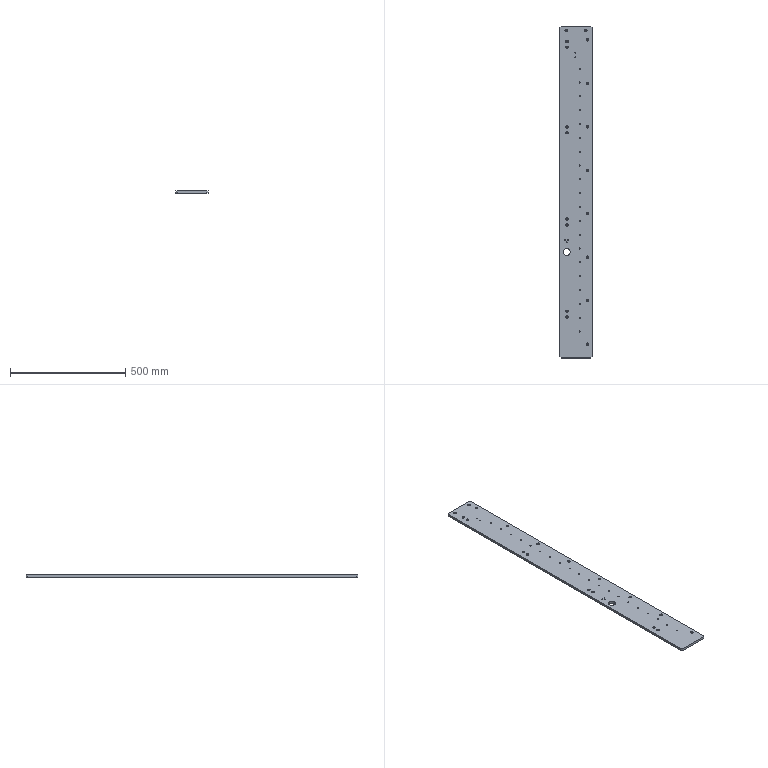Part | SolidWorks | features HoleWzd 5, Chamfer 1, Cut 1, Extrusion 1 | 1 solid | 152 faces | box 140 x 1440 x 10 mm | volume 1990912 mm3 | cylinder 124 | plane 28 | commonest cylinder face diameters 5 x40 6.6 x36 11 x36 3.3 x10 30 x2